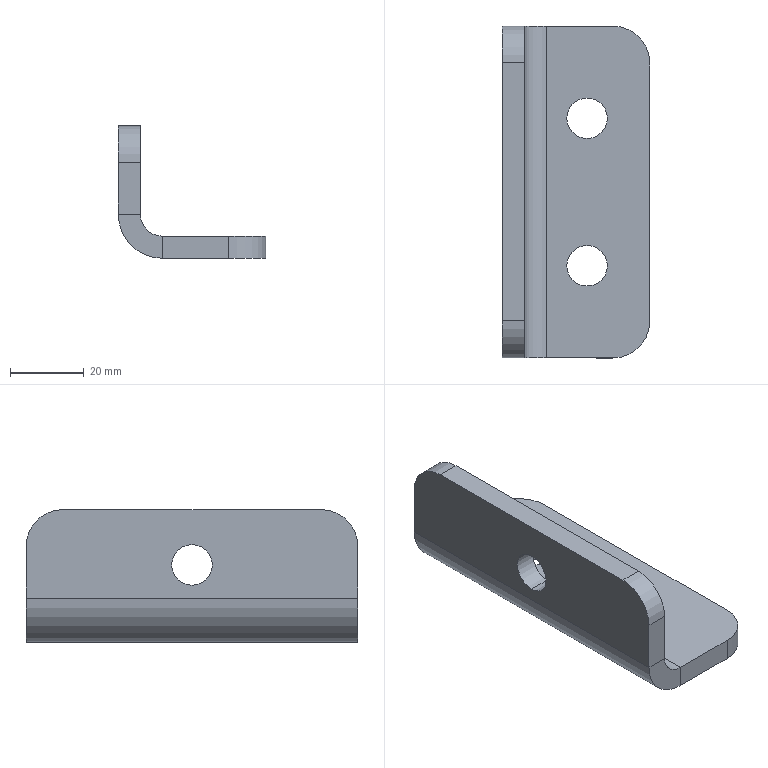Part | STEP file | Microwave Drying Flat Conveyor-CN2500x400-101-102 | 1 solid | 24 faces | box 40 x 90 x 36 mm | volume 33488 mm3 | cylinder 12 | plane 12 | commonest cylinder face diameters 11 x6 20 x4 12 x1 24 x1
STEP:
#1=CARTESIAN_POINT('',(-2.5,20.,-6.));
#2=VERTEX_POINT('',#1);
#3=CARTESIAN_POINT('',(8.5,20.,-6.));
#4=VERTEX_POINT('',#3);
#5=CARTESIAN_POINT('',(3.,20.,-6.));
#6=DIRECTION('',(0.,0.,1.));
#7=DIRECTION('',(1.,0.,0.));
#8=AXIS2_PLACEMENT_3D('',#5,#6,#7);
#9=CIRCLE('',#8,5.5);
#10=EDGE_CURVE('',#2,#4,#9,.T.);
#11=ORIENTED_EDGE('',*,*,#10,.F.);
#12=CARTESIAN_POINT('',(-2.5,20.,0.));
#13=VERTEX_POINT('',#12);
#14=CARTESIAN_POINT('',(-2.5,20.,-10.));
#15=DIRECTION('',(0.,0.,1.));
#16=VECTOR('',#15,1000.);
#17=LINE('',#14,#16);
#18=EDGE_CURVE('',#2,#13,#17,.T.);
#19=ORIENTED_EDGE('',*,*,#18,.T.);
#20=CARTESIAN_POINT('',(8.5,20.,0.));
#21=VERTEX_POINT('',#20);
#22=CARTESIAN_POINT('',(3.,20.,0.));
#23=DIRECTION('',(0.,0.,1.));
#24=DIRECTION('',(1.,0.,0.));
#25=AXIS2_PLACEMENT_3D('',#22,#23,#24);
#26=CIRCLE('',#25,5.5);
#27=EDGE_CURVE('',#13,#21,#26,.T.);
#28=ORIENTED_EDGE('',*,*,#27,.T.);
#29=CARTESIAN_POINT('',(8.5,20.,-10.));
#30=DIRECTION('',(0.,0.,1.));
#31=VECTOR('',#30,1000.);
#32=LINE('',#29,#31);
#33=EDGE_CURVE('',#4,#21,#32,.T.);
#34=ORIENTED_EDGE('',*,*,#33,.F.);
#35=EDGE_LOOP('',(#11,#19,#28,#34));
#36=FACE_OUTER_BOUND('',#35,.T.);
#37=CARTESIAN_POINT('',(3.,20.,-10.));
#38=DIRECTION('',(0.,0.,1.));
#39=DIRECTION('',(1.,0.,0.));
#40=AXIS2_PLACEMENT_3D('',#37,#38,#39);
#41=CYLINDRICAL_SURFACE('',#40,5.5);
#42=ADVANCED_FACE('',(#36),#41,.F.);
#43=CARTESIAN_POINT('',(-2.5,-20.,-6.));
#44=VERTEX_POINT('',#43);
#45=CARTESIAN_POINT('',(8.5,-20.,-6.));
#46=VERTEX_POINT('',#45);
#47=CARTESIAN_POINT('',(3.,-20.,-6.));
#48=DIRECTION('',(0.,0.,1.));
#49=DIRECTION('',(1.,0.,0.));
#50=AXIS2_PLACEMENT_3D('',#47,#48,#49);
#51=CIRCLE('',#50,5.5);
#52=EDGE_CURVE('',#44,#46,#51,.T.);
#53=ORIENTED_EDGE('',*,*,#52,.F.);
#54=CARTESIAN_POINT('',(-2.5,-20.,0.));
#55=VERTEX_POINT('',#54);
#56=CARTESIAN_POINT('',(-2.5,-20.,-10.));
#57=DIRECTION('',(0.,0.,1.));
#58=VECTOR('',#57,1000.);
#59=LINE('',#56,#58);
#60=EDGE_CURVE('',#44,#55,#59,.T.);
#61=ORIENTED_EDGE('',*,*,#60,.T.);
#62=CARTESIAN_POINT('',(8.5,-20.,0.));
#63=VERTEX_POINT('',#62);
#64=CARTESIAN_POINT('',(3.,-20.,0.));
#65=DIRECTION('',(0.,0.,1.));
#66=DIRECTION('',(1.,0.,0.));
#67=AXIS2_PLACEMENT_3D('',#64,#65,#66);
#68=CIRCLE('',#67,5.5);
#69=EDGE_CURVE('',#55,#63,#68,.T.);
#70=ORIENTED_EDGE('',*,*,#69,.T.);
#71=CARTESIAN_POINT('',(8.5,-20.,-10.));
#72=DIRECTION('',(0.,0.,1.));
#73=VECTOR('',#72,1000.);
#74=LINE('',#71,#73);
#75=EDGE_CURVE('',#46,#63,#74,.T.);
#76=ORIENTED_EDGE('',*,*,#75,.F.);
#77=EDGE_LOOP('',(#53,#61,#70,#76));
#78=FACE_OUTER_BOUND('',#77,.T.);
#79=CARTESIAN_POINT('',(3.,-20.,-10.));
#80=DIRECTION('',(0.,0.,1.));
#81=DIRECTION('',(1.,0.,0.));
#82=AXIS2_PLACEMENT_3D('',#79,#80,#81);
#83=CYLINDRICAL_SURFACE('',#82,5.5);
#84=ADVANCED_FACE('',(#78),#83,.F.);
#85=CARTESIAN_POINT('',(-14.,0.,20.5));
#86=VERTEX_POINT('',#85);
#87=CARTESIAN_POINT('',(-14.,0.,9.5));
#88=VERTEX_POINT('',#87);
#89=CARTESIAN_POINT('',(-14.,0.,15.));
#90=DIRECTION('',(1.,0.,0.));
#91=DIRECTION('',(0.,0.,-1.));
#92=AXIS2_PLACEMENT_3D('',#89,#90,#91);
#93=CIRCLE('',#92,5.5);
#94=EDGE_CURVE('',#86,#88,#93,.T.);
#95=ORIENTED_EDGE('',*,*,#94,.T.);
#96=CARTESIAN_POINT('',(-20.,0.,9.5));
#97=VERTEX_POINT('',#96);
#98=CARTESIAN_POINT('',(-10.,0.,9.5));
#99=DIRECTION('',(-1.,0.,0.));
#100=VECTOR('',#99,1000.);
#101=LINE('',#98,#100);
#102=EDGE_CURVE('',#88,#97,#101,.T.);
#103=ORIENTED_EDGE('',*,*,#102,.T.);
#104=CARTESIAN_POINT('',(-20.,0.,20.5));
#105=VERTEX_POINT('',#104);
#106=CARTESIAN_POINT('',(-20.,0.,15.));
#107=DIRECTION('',(-1.,0.,0.));
#108=DIRECTION('',(0.,0.,1.));
#109=AXIS2_PLACEMENT_3D('',#106,#107,#108);
#110=CIRCLE('',#109,5.5);
#111=EDGE_CURVE('',#97,#105,#110,.T.);
#112=ORIENTED_EDGE('',*,*,#111,.T.);
#113=CARTESIAN_POINT('',(-10.,0.,20.5));
#114=DIRECTION('',(-1.,0.,0.));
#115=VECTOR('',#114,1000.);
#116=LINE('',#113,#115);
#117=EDGE_CURVE('',#86,#105,#116,.T.);
#118=ORIENTED_EDGE('',*,*,#117,.F.);
#119=EDGE_LOOP('',(#95,#103,#112,#118));
#120=FACE_OUTER_BOUND('',#119,.T.);
#121=CARTESIAN_POINT('',(-10.,0.,15.));
#122=DIRECTION('',(-1.,0.,0.));
#123=DIRECTION('',(0.,0.,1.));
#124=AXIS2_PLACEMENT_3D('',#121,#122,#123);
#125=CYLINDRICAL_SURFACE('',#124,5.5);
#126=ADVANCED_FACE('',(#120),#125,.F.);
#127=CARTESIAN_POINT('',(-8.,-45.,0.));
#128=VERTEX_POINT('',#127);
#129=CARTESIAN_POINT('',(10.,-45.,0.));
#130=VERTEX_POINT('',#129);
#131=CARTESIAN_POINT('',(-20.,-45.,0.));
#132=DIRECTION('',(1.,0.,0.));
#133=VECTOR('',#132,1000.);
#134=LINE('',#131,#133);
#135=EDGE_CURVE('',#128,#130,#134,.T.);
#136=ORIENTED_EDGE('',*,*,#135,.F.);
#137=CARTESIAN_POINT('',(-8.,-45.,-6.));
#138=VERTEX_POINT('',#137);
#139=CARTESIAN_POINT('',(-8.,-45.,0.));
#140=DIRECTION('',(0.,0.,-1.));
#141=VECTOR('',#140,1000.);
#142=LINE('',#139,#141);
#143=EDGE_CURVE('',#128,#138,#142,.T.);
#144=ORIENTED_EDGE('',*,*,#143,.T.);
#145=CARTESIAN_POINT('',(10.,-45.,-6.));
#146=VERTEX_POINT('',#145);
#147=CARTESIAN_POINT('',(-20.,-45.,-6.));
#148=DIRECTION('',(1.,0.,0.));
#149=VECTOR('',#148,1000.);
#150=LINE('',#147,#149);
#151=EDGE_CURVE('',#138,#146,#150,.T.);
#152=ORIENTED_EDGE('',*,*,#151,.T.);
#153=CARTESIAN_POINT('',(10.,-45.,-6.));
#154=DIRECTION('',(0.,0.,1.));
#155=VECTOR('',#154,1000.);
#156=LINE('',#153,#155);
#157=EDGE_CURVE('',#146,#130,#156,.T.);
#158=ORIENTED_EDGE('',*,*,#157,.T.);
#159=EDGE_LOOP('',(#136,#144,#152,#158));
#160=FACE_OUTER_BOUND('',#159,.T.);
#161=CARTESIAN_POINT('',(-20.,-45.,-6.));
#162=DIRECTION('',(0.,-1.,0.));
#163=DIRECTION('',(0.,0.,-1.));
#164=AXIS2_PLACEMENT_3D('',#161,#162,#163);
#165=PLANE('',#164);
#166=ADVANCED_FACE('',(#160),#165,.T.);
#167=CARTESIAN_POINT('',(3.,20.,-6.));
#168=DIRECTION('',(0.,0.,1.));
#169=DIRECTION('',(1.,0.,0.));
#170=AXIS2_PLACEMENT_3D('',#167,#168,#169);
#171=CIRCLE('',#170,5.5);
#172=EDGE_CURVE('',#4,#2,#171,.T.);
#173=ORIENTED_EDGE('',*,*,#172,.T.);
#174=ORIENTED_EDGE('',*,*,#10,.T.);
#175=EDGE_LOOP('',(#173,#174));
#176=FACE_BOUND('',#175,.T.);
#177=CARTESIAN_POINT('',(3.,-20.,-6.));
#178=DIRECTION('',(0.,0.,1.));
#179=DIRECTION('',(1.,0.,0.));
#180=AXIS2_PLACEMENT_3D('',#177,#178,#179);
#181=CIRCLE('',#180,5.5);
#182=EDGE_CURVE('',#46,#44,#181,.T.);
#183=ORIENTED_EDGE('',*,*,#182,.T.);
#184=ORIENTED_EDGE('',*,*,#52,.T.);
#185=EDGE_LOOP('',(#183,#184));
#186=FACE_BOUND('',#185,.T.);
#187=CARTESIAN_POINT('',(-8.,45.,-6.));
#188=VERTEX_POINT('',#187);
#189=CARTESIAN_POINT('',(-8.,-45.,-6.));
#190=DIRECTION('',(0.,1.,0.));
#191=VECTOR('',#190,1000.);
#192=LINE('',#189,#191);
#193=EDGE_CURVE('',#138,#188,#192,.T.);
#194=ORIENTED_EDGE('',*,*,#193,.T.);
#195=CARTESIAN_POINT('',(10.,45.,-6.));
#196=VERTEX_POINT('',#195);
#197=CARTESIAN_POINT('',(-20.,45.,-6.));
#198=DIRECTION('',(-1.,0.,0.));
#199=VECTOR('',#198,1000.);
#200=LINE('',#197,#199);
#201=EDGE_CURVE('',#196,#188,#200,.T.);
#202=ORIENTED_EDGE('',*,*,#201,.F.);
#203=CARTESIAN_POINT('',(20.,35.,-6.));
#204=VERTEX_POINT('',#203);
#205=CARTESIAN_POINT('',(10.,35.,-6.));
#206=DIRECTION('',(0.,0.,1.));
#207=DIRECTION('',(-1.,0.,0.));
#208=AXIS2_PLACEMENT_3D('',#205,#206,#207);
#209=CIRCLE('',#208,10.);
#210=EDGE_CURVE('',#204,#196,#209,.T.);
#211=ORIENTED_EDGE('',*,*,#210,.F.);
#212=CARTESIAN_POINT('',(20.,-35.,-6.));
#213=VERTEX_POINT('',#212);
#214=CARTESIAN_POINT('',(20.,35.,-6.));
#215=DIRECTION('',(0.,1.,0.));
#216=VECTOR('',#215,1000.);
#217=LINE('',#214,#216);
#218=EDGE_CURVE('',#213,#204,#217,.T.);
#219=ORIENTED_EDGE('',*,*,#218,.F.);
#220=CARTESIAN_POINT('',(10.,-35.,-6.));
#221=DIRECTION('',(0.,0.,1.));
#222=DIRECTION('',(1.,0.,0.));
#223=AXIS2_PLACEMENT_3D('',#220,#221,#222);
#224=CIRCLE('',#223,10.);
#225=EDGE_CURVE('',#146,#213,#224,.T.);
#226=ORIENTED_EDGE('',*,*,#225,.F.);
#227=ORIENTED_EDGE('',*,*,#151,.F.);
#228=EDGE_LOOP('',(#194,#202,#211,#219,#226,#227));
#229=FACE_OUTER_BOUND('',#228,.T.);
#230=CARTESIAN_POINT('',(10.,-35.,-6.));
#231=DIRECTION('',(0.,0.,1.));
#232=DIRECTION('',(1.,0.,0.));
#233=AXIS2_PLACEMENT_3D('',#230,#231,#232);
#234=PLANE('',#233);
#235=ADVANCED_FACE('',(#176,#186,#229),#234,.F.);
#236=CARTESIAN_POINT('',(3.,20.,0.));
#237=DIRECTION('',(0.,0.,1.));
#238=DIRECTION('',(1.,0.,0.));
#239=AXIS2_PLACEMENT_3D('',#236,#237,#238);
#240=CIRCLE('',#239,5.5);
#241=EDGE_CURVE('',#21,#13,#240,.T.);
#242=ORIENTED_EDGE('',*,*,#241,.F.);
#243=ORIENTED_EDGE('',*,*,#27,.F.);
#244=EDGE_LOOP('',(#242,#243));
#245=FACE_BOUND('',#244,.T.);
#246=CARTESIAN_POINT('',(3.,-20.,0.));
#247=DIRECTION('',(0.,0.,1.));
#248=DIRECTION('',(1.,0.,0.));
#249=AXIS2_PLACEMENT_3D('',#246,#247,#248);
#250=CIRCLE('',#249,5.5);
#251=EDGE_CURVE('',#63,#55,#250,.T.);
#252=ORIENTED_EDGE('',*,*,#251,.F.);
#253=ORIENTED_EDGE('',*,*,#69,.F.);
#254=EDGE_LOOP('',(#252,#253));
#255=FACE_BOUND('',#254,.T.);
#256=CARTESIAN_POINT('',(10.,45.,0.));
#257=VERTEX_POINT('',#256);
#258=CARTESIAN_POINT('',(-8.,45.,0.));
#259=VERTEX_POINT('',#258);
#260=CARTESIAN_POINT('',(-20.,45.,0.));
#261=DIRECTION('',(-1.,0.,0.));
#262=VECTOR('',#261,1000.);
#263=LINE('',#260,#262);
#264=EDGE_CURVE('',#257,#259,#263,.T.);
#265=ORIENTED_EDGE('',*,*,#264,.T.);
#266=CARTESIAN_POINT('',(-8.,-45.,0.));
#267=DIRECTION('',(0.,1.,0.));
#268=VECTOR('',#267,1000.);
#269=LINE('',#266,#268);
#270=EDGE_CURVE('',#128,#259,#269,.T.);
#271=ORIENTED_EDGE('',*,*,#270,.F.);
#272=ORIENTED_EDGE('',*,*,#135,.T.);
#273=CARTESIAN_POINT('',(20.,-35.,0.));
#274=VERTEX_POINT('',#273);
#275=CARTESIAN_POINT('',(10.,-35.,0.));
#276=DIRECTION('',(0.,0.,1.));
#277=DIRECTION('',(1.,0.,0.));
#278=AXIS2_PLACEMENT_3D('',#275,#276,#277);
#279=CIRCLE('',#278,10.);
#280=EDGE_CURVE('',#130,#274,#279,.T.);
#281=ORIENTED_EDGE('',*,*,#280,.T.);
#282=CARTESIAN_POINT('',(20.,35.,0.));
#283=VERTEX_POINT('',#282);
#284=CARTESIAN_POINT('',(20.,35.,0.));
#285=DIRECTION('',(0.,1.,0.));
#286=VECTOR('',#285,1000.);
#287=LINE('',#284,#286);
#288=EDGE_CURVE('',#274,#283,#287,.T.);
#289=ORIENTED_EDGE('',*,*,#288,.T.);
#290=CARTESIAN_POINT('',(10.,35.,0.));
#291=DIRECTION('',(0.,0.,1.));
#292=DIRECTION('',(-1.,0.,0.));
#293=AXIS2_PLACEMENT_3D('',#290,#291,#292);
#294=CIRCLE('',#293,10.);
#295=EDGE_CURVE('',#283,#257,#294,.T.);
#296=ORIENTED_EDGE('',*,*,#295,.T.);
#297=EDGE_LOOP('',(#265,#271,#272,#281,#289,#296));
#298=FACE_OUTER_BOUND('',#297,.T.);
#299=CARTESIAN_POINT('',(10.,-35.,0.));
#300=DIRECTION('',(0.,0.,1.));
#301=DIRECTION('',(1.,0.,0.));
#302=AXIS2_PLACEMENT_3D('',#299,#300,#301);
#303=PLANE('',#302);
#304=ADVANCED_FACE('',(#245,#255,#298),#303,.T.);
#305=CARTESIAN_POINT('',(-8.,45.,0.));
#306=DIRECTION('',(0.,0.,-1.));
#307=VECTOR('',#306,1000.);
#308=LINE('',#305,#307);
#309=EDGE_CURVE('',#259,#188,#308,.T.);
#310=ORIENTED_EDGE('',*,*,#309,.F.);
#311=ORIENTED_EDGE('',*,*,#264,.F.);
#312=CARTESIAN_POINT('',(10.,45.,-6.));
#313=DIRECTION('',(0.,0.,1.));
#314=VECTOR('',#313,1000.);
#315=LINE('',#312,#314);
#316=EDGE_CURVE('',#196,#257,#315,.T.);
#317=ORIENTED_EDGE('',*,*,#316,.F.);
#318=ORIENTED_EDGE('',*,*,#201,.T.);
#319=EDGE_LOOP('',(#310,#311,#317,#318));
#320=FACE_OUTER_BOUND('',#319,.T.);
#321=CARTESIAN_POINT('',(-20.,45.,-6.));
#322=DIRECTION('',(0.,1.,0.));
#323=DIRECTION('',(0.,0.,1.));
#324=AXIS2_PLACEMENT_3D('',#321,#322,#323);
#325=PLANE('',#324);
#326=ADVANCED_FACE('',(#320),#325,.T.);
#327=ORIENTED_EDGE('',*,*,#295,.F.);
#328=CARTESIAN_POINT('',(20.,35.,-6.));
#329=DIRECTION('',(0.,0.,1.));
#330=VECTOR('',#329,1000.);
#331=LINE('',#328,#330);
#332=EDGE_CURVE('',#204,#283,#331,.T.);
#333=ORIENTED_EDGE('',*,*,#332,.F.);
#334=ORIENTED_EDGE('',*,*,#210,.T.);
#335=ORIENTED_EDGE('',*,*,#316,.T.);
#336=EDGE_LOOP('',(#327,#333,#334,#335));
#337=FACE_OUTER_BOUND('',#336,.T.);
#338=CARTESIAN_POINT('',(10.,35.,-6.));
#339=DIRECTION('',(0.,0.,1.));
#340=DIRECTION('',(1.,0.,0.));
#341=AXIS2_PLACEMENT_3D('',#338,#339,#340);
#342=CYLINDRICAL_SURFACE('',#341,10.);
#343=ADVANCED_FACE('',(#337),#342,.T.);
#344=ORIENTED_EDGE('',*,*,#288,.F.);
#345=CARTESIAN_POINT('',(20.,-35.,-6.));
#346=DIRECTION('',(0.,0.,1.));
#347=VECTOR('',#346,1000.);
#348=LINE('',#345,#347);
#349=EDGE_CURVE('',#213,#274,#348,.T.);
#350=ORIENTED_EDGE('',*,*,#349,.F.);
#351=ORIENTED_EDGE('',*,*,#218,.T.);
#352=ORIENTED_EDGE('',*,*,#332,.T.);
#353=EDGE_LOOP('',(#344,#350,#351,#352));
#354=FACE_OUTER_BOUND('',#353,.T.);
#355=CARTESIAN_POINT('',(20.,35.,-6.));
#356=DIRECTION('',(1.,0.,0.));
#357=DIRECTION('',(0.,1.,0.));
#358=AXIS2_PLACEMENT_3D('',#355,#356,#357);
#359=PLANE('',#358);
#360=ADVANCED_FACE('',(#354),#359,.T.);
#361=ORIENTED_EDGE('',*,*,#280,.F.);
#362=ORIENTED_EDGE('',*,*,#157,.F.);
#363=ORIENTED_EDGE('',*,*,#225,.T.);
#364=ORIENTED_EDGE('',*,*,#349,.T.);
#365=EDGE_LOOP('',(#361,#362,#363,#364));
#366=FACE_OUTER_BOUND('',#365,.T.);
#367=CARTESIAN_POINT('',(10.,-35.,-6.));
#368=DIRECTION('',(0.,0.,1.));
#369=DIRECTION('',(1.,0.,0.));
#370=AXIS2_PLACEMENT_3D('',#367,#368,#369);
#371=CYLINDRICAL_SURFACE('',#370,10.);
#372=ADVANCED_FACE('',(#366),#371,.T.);
#373=CARTESIAN_POINT('',(-14.,45.,6.));
#374=VERTEX_POINT('',#373);
#375=CARTESIAN_POINT('',(-20.,45.,6.));
#376=VERTEX_POINT('',#375);
#377=CARTESIAN_POINT('',(-20.,45.,6.));
#378=DIRECTION('',(-1.,0.,0.));
#379=VECTOR('',#378,1000.);
#380=LINE('',#377,#379);
#381=EDGE_CURVE('',#374,#376,#380,.T.);
#382=ORIENTED_EDGE('',*,*,#381,.F.);
#383=CARTESIAN_POINT('',(-8.,45.,6.));
#384=DIRECTION('',(0.,1.,0.));
#385=DIRECTION('',(1.,0.,0.));
#386=AXIS2_PLACEMENT_3D('',#383,#384,#385);
#387=CIRCLE('',#386,6.);
#388=EDGE_CURVE('',#259,#374,#387,.T.);
#389=ORIENTED_EDGE('',*,*,#388,.F.);
#390=ORIENTED_EDGE('',*,*,#309,.T.);
#391=CARTESIAN_POINT('',(-8.,45.,6.));
#392=DIRECTION('',(0.,1.,0.));
#393=DIRECTION('',(1.,0.,0.));
#394=AXIS2_PLACEMENT_3D('',#391,#392,#393);
#395=CIRCLE('',#394,12.);
#396=EDGE_CURVE('',#188,#376,#395,.T.);
#397=ORIENTED_EDGE('',*,*,#396,.T.);
#398=EDGE_LOOP('',(#382,#389,#390,#397));
#399=FACE_OUTER_BOUND('',#398,.T.);
#400=CARTESIAN_POINT('',(-8.,45.,6.));
#401=DIRECTION('',(0.,1.,0.));
#402=DIRECTION('',(-1.,0.,0.));
#403=AXIS2_PLACEMENT_3D('',#400,#401,#402);
#404=PLANE('',#403);
#405=ADVANCED_FACE('',(#399),#404,.T.);
#406=CARTESIAN_POINT('',(-14.,-45.,6.));
#407=VERTEX_POINT('',#406);
#408=CARTESIAN_POINT('',(-8.,-45.,6.));
#409=DIRECTION('',(0.,-1.,0.));
#410=DIRECTION('',(1.,0.,0.));
#411=AXIS2_PLACEMENT_3D('',#408,#409,#410);
#412=CIRCLE('',#411,6.);
#413=EDGE_CURVE('',#407,#128,#412,.T.);
#414=ORIENTED_EDGE('',*,*,#413,.F.);
#415=CARTESIAN_POINT('',(-20.,-45.,6.));
#416=VERTEX_POINT('',#415);
#417=CARTESIAN_POINT('',(-14.,-45.,6.));
#418=DIRECTION('',(-1.,0.,0.));
#419=VECTOR('',#418,1000.);
#420=LINE('',#417,#419);
#421=EDGE_CURVE('',#407,#416,#420,.T.);
#422=ORIENTED_EDGE('',*,*,#421,.T.);
#423=CARTESIAN_POINT('',(-8.,-45.,6.));
#424=DIRECTION('',(0.,-1.,0.));
#425=DIRECTION('',(1.,0.,0.));
#426=AXIS2_PLACEMENT_3D('',#423,#424,#425);
#427=CIRCLE('',#426,12.);
#428=EDGE_CURVE('',#416,#138,#427,.T.);
#429=ORIENTED_EDGE('',*,*,#428,.T.);
#430=ORIENTED_EDGE('',*,*,#143,.F.);
#431=EDGE_LOOP('',(#414,#422,#429,#430));
#432=FACE_OUTER_BOUND('',#431,.T.);
#433=CARTESIAN_POINT('',(-8.,-45.,6.));
#434=DIRECTION('',(0.,1.,0.));
#435=DIRECTION('',(-1.,0.,0.));
#436=AXIS2_PLACEMENT_3D('',#433,#434,#435);
#437=PLANE('',#436);
#438=ADVANCED_FACE('',(#432),#437,.F.);
#439=ORIENTED_EDGE('',*,*,#193,.F.);
#440=ORIENTED_EDGE('',*,*,#428,.F.);
#441=CARTESIAN_POINT('',(-20.,45.,6.));
#442=DIRECTION('',(0.,1.,0.));
#443=VECTOR('',#442,1000.);
#444=LINE('',#441,#443);
#445=EDGE_CURVE('',#416,#376,#444,.T.);
#446=ORIENTED_EDGE('',*,*,#445,.T.);
#447=ORIENTED_EDGE('',*,*,#396,.F.);
#448=EDGE_LOOP('',(#439,#440,#446,#447));
#449=FACE_OUTER_BOUND('',#448,.T.);
#450=CARTESIAN_POINT('',(-8.,-45.,6.));
#451=DIRECTION('',(0.,-1.,0.));
#452=DIRECTION('',(-1.,0.,0.));
#453=AXIS2_PLACEMENT_3D('',#450,#451,#452);
#454=CYLINDRICAL_SURFACE('',#453,12.);
#455=ADVANCED_FACE('',(#449),#454,.T.);
#456=ORIENTED_EDGE('',*,*,#270,.T.);
#457=ORIENTED_EDGE('',*,*,#388,.T.);
#458=CARTESIAN_POINT('',(-14.,45.,6.));
#459=DIRECTION('',(0.,-1.,0.));
#460=VECTOR('',#459,1000.);
#461=LINE('',#458,#460);
#462=EDGE_CURVE('',#374,#407,#461,.T.);
#463=ORIENTED_EDGE('',*,*,#462,.T.);
#464=ORIENTED_EDGE('',*,*,#413,.T.);
#465=EDGE_LOOP('',(#456,#457,#463,#464));
#466=FACE_OUTER_BOUND('',#465,.T.);
#467=CARTESIAN_POINT('',(-8.,-45.,6.));
#468=DIRECTION('',(0.,-1.,0.));
#469=DIRECTION('',(-1.,0.,0.));
#470=AXIS2_PLACEMENT_3D('',#467,#468,#469);
#471=CYLINDRICAL_SURFACE('',#470,6.);
#472=ADVANCED_FACE('',(#466),#471,.F.);
#473=ORIENTED_EDGE('',*,*,#381,.T.);
#474=CARTESIAN_POINT('',(-20.,45.,20.));
#475=VERTEX_POINT('',#474);
#476=CARTESIAN_POINT('',(-20.,45.,20.));
#477=DIRECTION('',(0.,0.,-1.));
#478=VECTOR('',#477,1000.);
#479=LINE('',#476,#478);
#480=EDGE_CURVE('',#475,#376,#479,.T.);
#481=ORIENTED_EDGE('',*,*,#480,.F.);
#482=CARTESIAN_POINT('',(-14.,45.,20.));
#483=VERTEX_POINT('',#482);
#484=CARTESIAN_POINT('',(-20.,45.,20.));
#485=DIRECTION('',(1.,0.,0.));
#486=VECTOR('',#485,1000.);
#487=LINE('',#484,#486);
#488=EDGE_CURVE('',#475,#483,#487,.T.);
#489=ORIENTED_EDGE('',*,*,#488,.T.);
#490=CARTESIAN_POINT('',(-14.,45.,0.));
#491=DIRECTION('',(0.,0.,-1.));
#492=VECTOR('',#491,1000.);
#493=LINE('',#490,#492);
#494=EDGE_CURVE('',#483,#374,#493,.T.);
#495=ORIENTED_EDGE('',*,*,#494,.T.);
#496=EDGE_LOOP('',(#473,#481,#489,#495));
#497=FACE_OUTER_BOUND('',#496,.T.);
#498=CARTESIAN_POINT('',(-20.,45.,0.));
#499=DIRECTION('',(0.,-1.,0.));
#500=DIRECTION('',(0.,0.,-1.));
#501=AXIS2_PLACEMENT_3D('',#498,#499,#500);
#502=PLANE('',#501);
#503=ADVANCED_FACE('',(#497),#502,.F.);
#504=ORIENTED_EDGE('',*,*,#421,.F.);
#505=CARTESIAN_POINT('',(-14.,-45.,20.));
#506=VERTEX_POINT('',#505);
#507=CARTESIAN_POINT('',(-14.,-45.,20.));
#508=DIRECTION('',(0.,0.,1.));
#509=VECTOR('',#508,1000.);
#510=LINE('',#507,#509);
#511=EDGE_CURVE('',#407,#506,#510,.T.);
#512=ORIENTED_EDGE('',*,*,#511,.T.);
#513=CARTESIAN_POINT('',(-20.,-45.,20.));
#514=VERTEX_POINT('',#513);
#515=CARTESIAN_POINT('',(-20.,-45.,20.));
#516=DIRECTION('',(1.,0.,0.));
#517=VECTOR('',#516,1000.);
#518=LINE('',#515,#517);
#519=EDGE_CURVE('',#514,#506,#518,.T.);
#520=ORIENTED_EDGE('',*,*,#519,.F.);
#521=CARTESIAN_POINT('',(-20.,-45.,20.));
#522=DIRECTION('',(0.,0.,1.));
#523=VECTOR('',#522,1000.);
#524=LINE('',#521,#523);
#525=EDGE_CURVE('',#416,#514,#524,.T.);
#526=ORIENTED_EDGE('',*,*,#525,.F.);
#527=EDGE_LOOP('',(#504,#512,#520,#526));
#528=FACE_OUTER_BOUND('',#527,.T.);
#529=CARTESIAN_POINT('',(-20.,-45.,20.));
#530=DIRECTION('',(0.,1.,0.));
#531=DIRECTION('',(0.,0.,1.));
#532=AXIS2_PLACEMENT_3D('',#529,#530,#531);
#533=PLANE('',#532);
#534=ADVANCED_FACE('',(#528),#533,.F.);
#535=CARTESIAN_POINT('',(-20.,0.,15.));
#536=DIRECTION('',(-1.,0.,0.));
#537=DIRECTION('',(0.,0.,1.));
#538=AXIS2_PLACEMENT_3D('',#535,#536,#537);
#539=CIRCLE('',#538,5.5);
#540=EDGE_CURVE('',#105,#97,#539,.T.);
#541=ORIENTED_EDGE('',*,*,#540,.F.);
#542=ORIENTED_EDGE('',*,*,#111,.F.);
#543=EDGE_LOOP('',(#541,#542));
#544=FACE_BOUND('',#543,.T.);
#545=ORIENTED_EDGE('',*,*,#445,.F.);
#546=ORIENTED_EDGE('',*,*,#525,.T.);
#547=CARTESIAN_POINT('',(-20.,-35.,30.));
#548=VERTEX_POINT('',#547);
#549=CARTESIAN_POINT('',(-20.,-35.,20.));
#550=DIRECTION('',(-1.,0.,0.));
#551=DIRECTION('',(0.,0.,-1.));
#552=AXIS2_PLACEMENT_3D('',#549,#550,#551);
#553=CIRCLE('',#552,10.);
#554=EDGE_CURVE('',#514,#548,#553,.T.);
#555=ORIENTED_EDGE('',*,*,#554,.T.);
#556=CARTESIAN_POINT('',(-20.,35.,30.));
#557=VERTEX_POINT('',#556);
#558=CARTESIAN_POINT('',(-20.,35.,30.));
#559=DIRECTION('',(0.,1.,0.));
#560=VECTOR('',#559,1000.);
#561=LINE('',#558,#560);
#562=EDGE_CURVE('',#548,#557,#561,.T.);
#563=ORIENTED_EDGE('',*,*,#562,.T.);
#564=CARTESIAN_POINT('',(-20.,35.,20.));
#565=DIRECTION('',(-1.,0.,0.));
#566=DIRECTION('',(0.,0.,-1.));
#567=AXIS2_PLACEMENT_3D('',#564,#565,#566);
#568=CIRCLE('',#567,10.);
#569=EDGE_CURVE('',#557,#475,#568,.T.);
#570=ORIENTED_EDGE('',*,*,#569,.T.);
#571=ORIENTED_EDGE('',*,*,#480,.T.);
#572=EDGE_LOOP('',(#545,#546,#555,#563,#570,#571));
#573=FACE_OUTER_BOUND('',#572,.T.);
#574=CARTESIAN_POINT('',(-20.,35.,20.));
#575=DIRECTION('',(1.,0.,0.));
#576=DIRECTION('',(0.,0.,-1.));
#577=AXIS2_PLACEMENT_3D('',#574,#575,#576);
#578=PLANE('',#577);
#579=ADVANCED_FACE('',(#544,#573),#578,.F.);
#580=ORIENTED_EDGE('',*,*,#94,.F.);
#581=CARTESIAN_POINT('',(-14.,0.,15.));
#582=DIRECTION('',(1.,0.,0.));
#583=DIRECTION('',(0.,0.,-1.));
#584=AXIS2_PLACEMENT_3D('',#581,#582,#583);
#585=CIRCLE('',#584,5.5);
#586=EDGE_CURVE('',#88,#86,#585,.T.);
#587=ORIENTED_EDGE('',*,*,#586,.F.);
#588=EDGE_LOOP('',(#580,#587));
#589=FACE_BOUND('',#588,.T.);
#590=ORIENTED_EDGE('',*,*,#511,.F.);
#591=ORIENTED_EDGE('',*,*,#462,.F.);
#592=ORIENTED_EDGE('',*,*,#494,.F.);
#593=CARTESIAN_POINT('',(-14.,35.,30.));
#594=VERTEX_POINT('',#593);
#595=CARTESIAN_POINT('',(-14.,35.,20.));
#596=DIRECTION('',(-1.,0.,0.));
#597=DIRECTION('',(0.,0.,-1.));
#598=AXIS2_PLACEMENT_3D('',#595,#596,#597);
#599=CIRCLE('',#598,10.);
#600=EDGE_CURVE('',#594,#483,#599,.T.);
#601=ORIENTED_EDGE('',*,*,#600,.F.);
#602=CARTESIAN_POINT('',(-14.,-35.,30.));
#603=VERTEX_POINT('',#602);
#604=CARTESIAN_POINT('',(-14.,35.,30.));
#605=DIRECTION('',(0.,1.,0.));
#606=VECTOR('',#605,1000.);
#607=LINE('',#604,#606);
#608=EDGE_CURVE('',#603,#594,#607,.T.);
#609=ORIENTED_EDGE('',*,*,#608,.F.);
#610=CARTESIAN_POINT('',(-14.,-35.,20.));
#611=DIRECTION('',(-1.,0.,0.));
#612=DIRECTION('',(0.,0.,-1.));
#613=AXIS2_PLACEMENT_3D('',#610,#611,#612);
#614=CIRCLE('',#613,10.);
#615=EDGE_CURVE('',#506,#603,#614,.T.);
#616=ORIENTED_EDGE('',*,*,#615,.F.);
#617=EDGE_LOOP('',(#590,#591,#592,#601,#609,#616));
#618=FACE_OUTER_BOUND('',#617,.T.);
#619=CARTESIAN_POINT('',(-14.,35.,20.));
#620=DIRECTION('',(1.,0.,0.));
#621=DIRECTION('',(0.,0.,-1.));
#622=AXIS2_PLACEMENT_3D('',#619,#620,#621);
#623=PLANE('',#622);
#624=ADVANCED_FACE('',(#589,#618),#623,.T.);
#625=ORIENTED_EDGE('',*,*,#615,.T.);
#626=CARTESIAN_POINT('',(-20.,-35.,30.));
#627=DIRECTION('',(1.,0.,0.));
#628=VECTOR('',#627,1000.);
#629=LINE('',#626,#628);
#630=EDGE_CURVE('',#548,#603,#629,.T.);
#631=ORIENTED_EDGE('',*,*,#630,.F.);
#632=ORIENTED_EDGE('',*,*,#554,.F.);
#633=ORIENTED_EDGE('',*,*,#519,.T.);
#634=EDGE_LOOP('',(#625,#631,#632,#633));
#635=FACE_OUTER_BOUND('',#634,.T.);
#636=CARTESIAN_POINT('',(-20.,-35.,20.));
#637=DIRECTION('',(1.,0.,0.));
#638=DIRECTION('',(0.,0.,-1.));
#639=AXIS2_PLACEMENT_3D('',#636,#637,#638);
#640=CYLINDRICAL_SURFACE('',#639,10.);
#641=ADVANCED_FACE('',(#635),#640,.T.);
#642=ORIENTED_EDGE('',*,*,#608,.T.);
#643=CARTESIAN_POINT('',(-20.,35.,30.));
#644=DIRECTION('',(1.,0.,0.));
#645=VECTOR('',#644,1000.);
#646=LINE('',#643,#645);
#647=EDGE_CURVE('',#557,#594,#646,.T.);
#648=ORIENTED_EDGE('',*,*,#647,.F.);
#649=ORIENTED_EDGE('',*,*,#562,.F.);
#650=ORIENTED_EDGE('',*,*,#630,.T.);
#651=EDGE_LOOP('',(#642,#648,#649,#650));
#652=FACE_OUTER_BOUND('',#651,.T.);
#653=CARTESIAN_POINT('',(-20.,35.,30.));
#654=DIRECTION('',(0.,0.,-1.));
#655=DIRECTION('',(-1.,0.,0.));
#656=AXIS2_PLACEMENT_3D('',#653,#654,#655);
#657=PLANE('',#656);
#658=ADVANCED_FACE('',(#652),#657,.F.);
#659=ORIENTED_EDGE('',*,*,#600,.T.);
#660=ORIENTED_EDGE('',*,*,#488,.F.);
#661=ORIENTED_EDGE('',*,*,#569,.F.);
#662=ORIENTED_EDGE('',*,*,#647,.T.);
#663=EDGE_LOOP('',(#659,#660,#661,#662));
#664=FACE_OUTER_BOUND('',#663,.T.);
#665=CARTESIAN_POINT('',(-20.,35.,20.));
#666=DIRECTION('',(1.,0.,0.));
#667=DIRECTION('',(0.,0.,-1.));
#668=AXIS2_PLACEMENT_3D('',#665,#666,#667);
#669=CYLINDRICAL_SURFACE('',#668,10.);
#670=ADVANCED_FACE('',(#664),#669,.T.);
#671=ORIENTED_EDGE('',*,*,#102,.F.);
#672=ORIENTED_EDGE('',*,*,#586,.T.);
#673=ORIENTED_EDGE('',*,*,#117,.T.);
#674=ORIENTED_EDGE('',*,*,#540,.T.);
#675=EDGE_LOOP('',(#671,#672,#673,#674));
#676=FACE_OUTER_BOUND('',#675,.T.);
#677=CARTESIAN_POINT('',(-10.,0.,15.));
#678=DIRECTION('',(-1.,0.,0.));
#679=DIRECTION('',(0.,0.,1.));
#680=AXIS2_PLACEMENT_3D('',#677,#678,#679);
#681=CYLINDRICAL_SURFACE('',#680,5.5);
#682=ADVANCED_FACE('',(#676),#681,.F.);
#683=ORIENTED_EDGE('',*,*,#60,.F.);
#684=ORIENTED_EDGE('',*,*,#182,.F.);
#685=ORIENTED_EDGE('',*,*,#75,.T.);
#686=ORIENTED_EDGE('',*,*,#251,.T.);
#687=EDGE_LOOP('',(#683,#684,#685,#686));
#688=FACE_OUTER_BOUND('',#687,.T.);
#689=CARTESIAN_POINT('',(3.,-20.,-10.));
#690=DIRECTION('',(0.,0.,1.));
#691=DIRECTION('',(1.,0.,0.));
#692=AXIS2_PLACEMENT_3D('',#689,#690,#691);
#693=CYLINDRICAL_SURFACE('',#692,5.5);
#694=ADVANCED_FACE('',(#688),#693,.F.);
#695=ORIENTED_EDGE('',*,*,#18,.F.);
#696=ORIENTED_EDGE('',*,*,#172,.F.);
#697=ORIENTED_EDGE('',*,*,#33,.T.);
#698=ORIENTED_EDGE('',*,*,#241,.T.);
#699=EDGE_LOOP('',(#695,#696,#697,#698));
#700=FACE_OUTER_BOUND('',#699,.T.);
#701=CARTESIAN_POINT('',(3.,20.,-10.));
#702=DIRECTION('',(0.,0.,1.));
#703=DIRECTION('',(1.,0.,0.));
#704=AXIS2_PLACEMENT_3D('',#701,#702,#703);
#705=CYLINDRICAL_SURFACE('',#704,5.5);
#706=ADVANCED_FACE('',(#700),#705,.F.);
#707=CLOSED_SHELL('',(#42,#84,#126,#166,#235,#304,#326,#343,#360,#372,#405,#438,#455,#472,#503,#534,#579,#624,#641,#658,#670,#682,#694,#706));
#708=MANIFOLD_SOLID_BREP('',#707);
#709=CARTESIAN_POINT('',(0.,0.,0.));
#710=DIRECTION('',(0.,0.,1.));
#711=DIRECTION('',(1.,0.,0.));
#712=AXIS2_PLACEMENT_3D('',#709,#710,#711);
#713=(LENGTH_UNIT()NAMED_UNIT(*)SI_UNIT(.MILLI.,.METRE.));
#714=UNCERTAINTY_MEASURE_WITH_UNIT(LENGTH_MEASURE(0.00001),#713,'','');
#715=(NAMED_UNIT(*)PLANE_ANGLE_UNIT()SI_UNIT($,.RADIAN.));
#716=(NAMED_UNIT(*)SI_UNIT($,.STERADIAN.)SOLID_ANGLE_UNIT());
#717=(GEOMETRIC_REPRESENTATION_CONTEXT(3)GLOBAL_UNCERTAINTY_ASSIGNED_CONTEXT((#714))GLOBAL_UNIT_ASSIGNED_CONTEXT((#713,#715,#716))REPRESENTATION_CONTEXT('',''));
#718=ADVANCED_BREP_SHAPE_REPRESENTATION('',(#708,#712),#717);